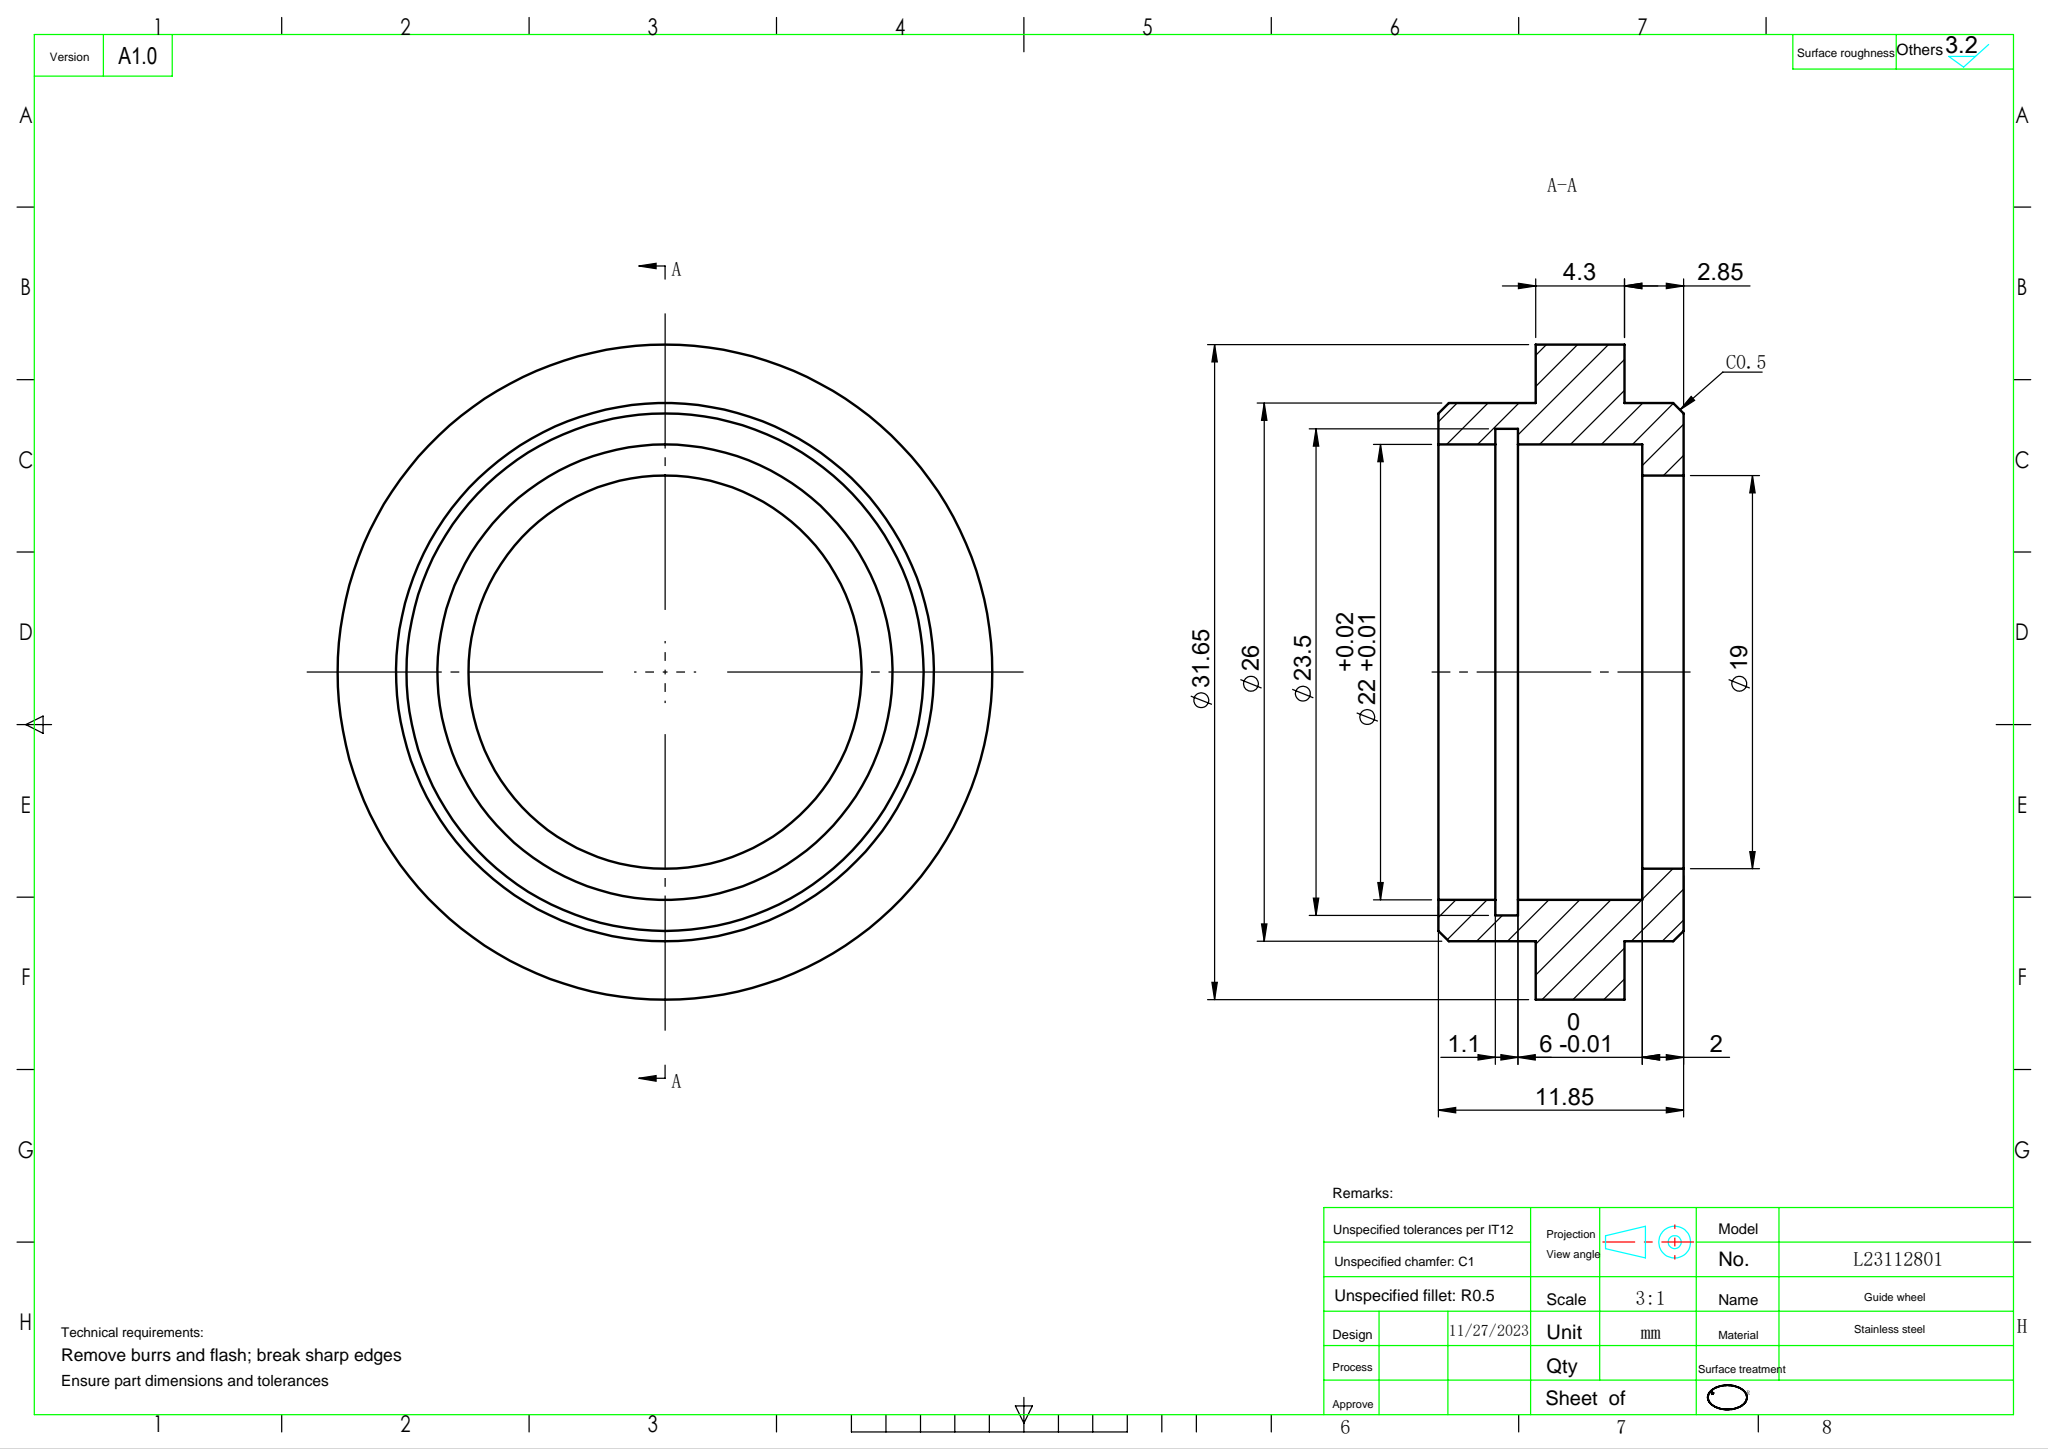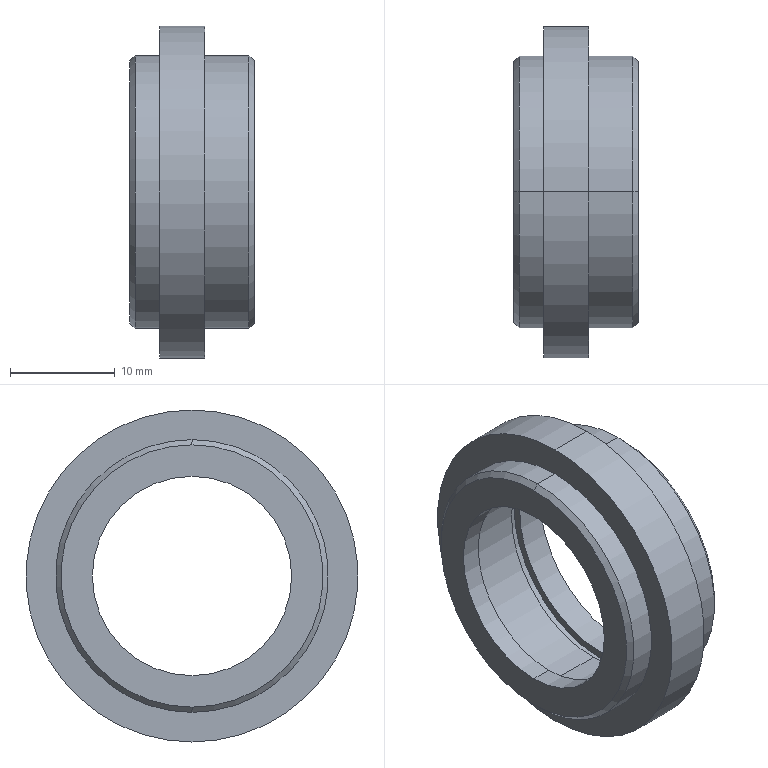Part | SolidWorks | features ICE 2, Chamfer 1, Revolution 1 | 1 solid | 25 faces | box 11.85 x 31.65 x 31.65 mm | volume 3001 mm3 | cylinder 14 | plane 7 | cone 4 | commonest cylinder face diameters 22 x4 26 x4 19 x2 23.5 x2 31.65 x2
STEP:
#1=CARTESIAN_POINT('',(0.,0.,12.5));
#2=VERTEX_POINT('',#1);
#3=CARTESIAN_POINT('',(0.,0.,-12.5));
#4=VERTEX_POINT('',#3);
#5=CARTESIAN_POINT('',(0.,0.,0.));
#6=DIRECTION('',(-1.,0.,0.));
#7=DIRECTION('',(0.,0.,-1.));
#8=AXIS2_PLACEMENT_3D('',#5,#6,#7);
#9=CIRCLE('',#8,12.5);
#10=EDGE_CURVE('',#2,#4,#9,.T.);
#11=ORIENTED_EDGE('',*,*,#10,.F.);
#12=CARTESIAN_POINT('',(0.5,0.,13.));
#13=VERTEX_POINT('',#12);
#14=CARTESIAN_POINT('',(0.,0.,12.5));
#15=DIRECTION('',(0.7071,0.,0.7071));
#16=VECTOR('',#15,1000.);
#17=LINE('',#14,#16);
#18=EDGE_CURVE('',#2,#13,#17,.T.);
#19=ORIENTED_EDGE('',*,*,#18,.T.);
#20=CARTESIAN_POINT('',(0.5,0.,-13.));
#21=VERTEX_POINT('',#20);
#22=CARTESIAN_POINT('',(0.5,0.,0.));
#23=DIRECTION('',(1.,0.,0.));
#24=DIRECTION('',(0.,0.,-1.));
#25=AXIS2_PLACEMENT_3D('',#22,#23,#24);
#26=CIRCLE('',#25,13.);
#27=EDGE_CURVE('',#21,#13,#26,.T.);
#28=ORIENTED_EDGE('',*,*,#27,.F.);
#29=CARTESIAN_POINT('',(0.,0.,-12.5));
#30=DIRECTION('',(0.7071,0.,-0.7071));
#31=VECTOR('',#30,1000.);
#32=LINE('',#29,#31);
#33=EDGE_CURVE('',#4,#21,#32,.T.);
#34=ORIENTED_EDGE('',*,*,#33,.F.);
#35=EDGE_LOOP('',(#11,#19,#28,#34));
#36=FACE_OUTER_BOUND('',#35,.T.);
#37=CARTESIAN_POINT('',(0.,0.,0.));
#38=DIRECTION('',(1.,0.,0.));
#39=DIRECTION('',(0.,0.,-1.));
#40=AXIS2_PLACEMENT_3D('',#37,#38,#39);
#41=CONICAL_SURFACE('',#40,12.5,0.7854);
#42=ADVANCED_FACE('',(#36),#41,.T.);
#43=CARTESIAN_POINT('',(11.85,0.,-12.5));
#44=VERTEX_POINT('',#43);
#45=CARTESIAN_POINT('',(11.85,0.,12.5));
#46=VERTEX_POINT('',#45);
#47=CARTESIAN_POINT('',(11.85,0.,0.));
#48=DIRECTION('',(1.,0.,0.));
#49=DIRECTION('',(0.,0.,1.));
#50=AXIS2_PLACEMENT_3D('',#47,#48,#49);
#51=CIRCLE('',#50,12.5);
#52=EDGE_CURVE('',#44,#46,#51,.T.);
#53=ORIENTED_EDGE('',*,*,#52,.F.);
#54=CARTESIAN_POINT('',(11.35,0.,-13.));
#55=VERTEX_POINT('',#54);
#56=CARTESIAN_POINT('',(11.35,0.,-13.));
#57=DIRECTION('',(-0.7071,0.,-0.7071));
#58=VECTOR('',#57,1000.);
#59=LINE('',#56,#58);
#60=EDGE_CURVE('',#44,#55,#59,.T.);
#61=ORIENTED_EDGE('',*,*,#60,.T.);
#62=CARTESIAN_POINT('',(11.35,0.,13.));
#63=VERTEX_POINT('',#62);
#64=CARTESIAN_POINT('',(11.35,0.,0.));
#65=DIRECTION('',(-1.,0.,0.));
#66=DIRECTION('',(0.,0.,1.));
#67=AXIS2_PLACEMENT_3D('',#64,#65,#66);
#68=CIRCLE('',#67,13.);
#69=EDGE_CURVE('',#63,#55,#68,.T.);
#70=ORIENTED_EDGE('',*,*,#69,.F.);
#71=CARTESIAN_POINT('',(11.35,0.,13.));
#72=DIRECTION('',(-0.7071,0.,0.7071));
#73=VECTOR('',#72,1000.);
#74=LINE('',#71,#73);
#75=EDGE_CURVE('',#46,#63,#74,.T.);
#76=ORIENTED_EDGE('',*,*,#75,.F.);
#77=EDGE_LOOP('',(#53,#61,#70,#76));
#78=FACE_OUTER_BOUND('',#77,.T.);
#79=CARTESIAN_POINT('',(11.35,0.,0.));
#80=DIRECTION('',(-1.,0.,0.));
#81=DIRECTION('',(0.,0.,1.));
#82=AXIS2_PLACEMENT_3D('',#79,#80,#81);
#83=CONICAL_SURFACE('',#82,13.,0.7854);
#84=ADVANCED_FACE('',(#78),#83,.T.);
#85=CARTESIAN_POINT('',(9.1,0.,11.75));
#86=VERTEX_POINT('',#85);
#87=CARTESIAN_POINT('',(9.1,0.,-11.75));
#88=VERTEX_POINT('',#87);
#89=CARTESIAN_POINT('',(9.1,0.,0.));
#90=DIRECTION('',(1.,0.,0.));
#91=DIRECTION('',(0.,0.,-1.));
#92=AXIS2_PLACEMENT_3D('',#89,#90,#91);
#93=CIRCLE('',#92,11.75);
#94=EDGE_CURVE('',#86,#88,#93,.T.);
#95=ORIENTED_EDGE('',*,*,#94,.T.);
#96=CARTESIAN_POINT('',(8.,0.,-11.75));
#97=VERTEX_POINT('',#96);
#98=CARTESIAN_POINT('',(9.1,0.,-11.75));
#99=DIRECTION('',(-1.,0.,0.));
#100=VECTOR('',#99,1000.);
#101=LINE('',#98,#100);
#102=EDGE_CURVE('',#88,#97,#101,.T.);
#103=ORIENTED_EDGE('',*,*,#102,.T.);
#104=CARTESIAN_POINT('',(8.,0.,11.75));
#105=VERTEX_POINT('',#104);
#106=CARTESIAN_POINT('',(8.,0.,0.));
#107=DIRECTION('',(1.,0.,0.));
#108=DIRECTION('',(0.,0.,-1.));
#109=AXIS2_PLACEMENT_3D('',#106,#107,#108);
#110=CIRCLE('',#109,11.75);
#111=EDGE_CURVE('',#105,#97,#110,.T.);
#112=ORIENTED_EDGE('',*,*,#111,.F.);
#113=CARTESIAN_POINT('',(9.1,0.,11.75));
#114=DIRECTION('',(-1.,0.,0.));
#115=VECTOR('',#114,1000.);
#116=LINE('',#113,#115);
#117=EDGE_CURVE('',#86,#105,#116,.T.);
#118=ORIENTED_EDGE('',*,*,#117,.F.);
#119=EDGE_LOOP('',(#95,#103,#112,#118));
#120=FACE_OUTER_BOUND('',#119,.T.);
#121=CARTESIAN_POINT('',(9.1,0.,0.));
#122=DIRECTION('',(-1.,0.,0.));
#123=DIRECTION('',(0.,0.,1.));
#124=AXIS2_PLACEMENT_3D('',#121,#122,#123);
#125=CYLINDRICAL_SURFACE('',#124,11.75);
#126=ADVANCED_FACE('',(#120),#125,.F.);
#127=CARTESIAN_POINT('',(11.85,0.,11.));
#128=VERTEX_POINT('',#127);
#129=CARTESIAN_POINT('',(11.85,0.,-11.));
#130=VERTEX_POINT('',#129);
#131=CARTESIAN_POINT('',(11.85,0.,0.));
#132=DIRECTION('',(1.,0.,0.));
#133=DIRECTION('',(0.,0.,-1.));
#134=AXIS2_PLACEMENT_3D('',#131,#132,#133);
#135=CIRCLE('',#134,11.);
#136=EDGE_CURVE('',#128,#130,#135,.T.);
#137=ORIENTED_EDGE('',*,*,#136,.T.);
#138=CARTESIAN_POINT('',(9.1,0.,-11.));
#139=VERTEX_POINT('',#138);
#140=CARTESIAN_POINT('',(11.85,0.,-11.));
#141=DIRECTION('',(-1.,0.,0.));
#142=VECTOR('',#141,1000.);
#143=LINE('',#140,#142);
#144=EDGE_CURVE('',#130,#139,#143,.T.);
#145=ORIENTED_EDGE('',*,*,#144,.T.);
#146=CARTESIAN_POINT('',(9.1,0.,11.));
#147=VERTEX_POINT('',#146);
#148=CARTESIAN_POINT('',(9.1,0.,0.));
#149=DIRECTION('',(1.,0.,0.));
#150=DIRECTION('',(0.,0.,-1.));
#151=AXIS2_PLACEMENT_3D('',#148,#149,#150);
#152=CIRCLE('',#151,11.);
#153=EDGE_CURVE('',#147,#139,#152,.T.);
#154=ORIENTED_EDGE('',*,*,#153,.F.);
#155=CARTESIAN_POINT('',(11.85,0.,11.));
#156=DIRECTION('',(-1.,0.,0.));
#157=VECTOR('',#156,1000.);
#158=LINE('',#155,#157);
#159=EDGE_CURVE('',#128,#147,#158,.T.);
#160=ORIENTED_EDGE('',*,*,#159,.F.);
#161=EDGE_LOOP('',(#137,#145,#154,#160));
#162=FACE_OUTER_BOUND('',#161,.T.);
#163=CARTESIAN_POINT('',(11.85,0.,0.));
#164=DIRECTION('',(-1.,0.,0.));
#165=DIRECTION('',(0.,0.,1.));
#166=AXIS2_PLACEMENT_3D('',#163,#164,#165);
#167=CYLINDRICAL_SURFACE('',#166,11.);
#168=ADVANCED_FACE('',(#162),#167,.F.);
#169=ORIENTED_EDGE('',*,*,#69,.T.);
#170=CARTESIAN_POINT('',(7.15,0.,-13.));
#171=VERTEX_POINT('',#170);
#172=CARTESIAN_POINT('',(0.,0.,-13.));
#173=DIRECTION('',(-1.,0.,0.));
#174=VECTOR('',#173,1000.);
#175=LINE('',#172,#174);
#176=EDGE_CURVE('',#55,#171,#175,.T.);
#177=ORIENTED_EDGE('',*,*,#176,.T.);
#178=CARTESIAN_POINT('',(7.15,0.,13.));
#179=VERTEX_POINT('',#178);
#180=CARTESIAN_POINT('',(7.15,0.,0.));
#181=DIRECTION('',(-1.,0.,0.));
#182=DIRECTION('',(0.,0.,1.));
#183=AXIS2_PLACEMENT_3D('',#180,#181,#182);
#184=CIRCLE('',#183,13.);
#185=EDGE_CURVE('',#179,#171,#184,.T.);
#186=ORIENTED_EDGE('',*,*,#185,.F.);
#187=CARTESIAN_POINT('',(0.,0.,13.));
#188=DIRECTION('',(-1.,0.,0.));
#189=VECTOR('',#188,1000.);
#190=LINE('',#187,#189);
#191=EDGE_CURVE('',#63,#179,#190,.T.);
#192=ORIENTED_EDGE('',*,*,#191,.F.);
#193=EDGE_LOOP('',(#169,#177,#186,#192));
#194=FACE_OUTER_BOUND('',#193,.T.);
#195=CARTESIAN_POINT('',(0.,0.,0.));
#196=DIRECTION('',(-1.,0.,0.));
#197=DIRECTION('',(0.,0.,1.));
#198=AXIS2_PLACEMENT_3D('',#195,#196,#197);
#199=CYLINDRICAL_SURFACE('',#198,13.);
#200=ADVANCED_FACE('',(#194),#199,.T.);
#201=CARTESIAN_POINT('',(7.15,0.,15.825));
#202=VERTEX_POINT('',#201);
#203=CARTESIAN_POINT('',(7.15,0.,-15.825));
#204=VERTEX_POINT('',#203);
#205=CARTESIAN_POINT('',(7.15,0.,0.));
#206=DIRECTION('',(-1.,0.,0.));
#207=DIRECTION('',(0.,0.,1.));
#208=AXIS2_PLACEMENT_3D('',#205,#206,#207);
#209=CIRCLE('',#208,15.825);
#210=EDGE_CURVE('',#202,#204,#209,.T.);
#211=ORIENTED_EDGE('',*,*,#210,.T.);
#212=CARTESIAN_POINT('',(2.85,0.,-15.825));
#213=VERTEX_POINT('',#212);
#214=CARTESIAN_POINT('',(0.,0.,-15.825));
#215=DIRECTION('',(-1.,0.,0.));
#216=VECTOR('',#215,1000.);
#217=LINE('',#214,#216);
#218=EDGE_CURVE('',#204,#213,#217,.T.);
#219=ORIENTED_EDGE('',*,*,#218,.T.);
#220=CARTESIAN_POINT('',(2.85,0.,15.825));
#221=VERTEX_POINT('',#220);
#222=CARTESIAN_POINT('',(2.85,0.,0.));
#223=DIRECTION('',(-1.,0.,0.));
#224=DIRECTION('',(0.,0.,1.));
#225=AXIS2_PLACEMENT_3D('',#222,#223,#224);
#226=CIRCLE('',#225,15.825);
#227=EDGE_CURVE('',#221,#213,#226,.T.);
#228=ORIENTED_EDGE('',*,*,#227,.F.);
#229=CARTESIAN_POINT('',(0.,0.,15.825));
#230=DIRECTION('',(-1.,0.,0.));
#231=VECTOR('',#230,1000.);
#232=LINE('',#229,#231);
#233=EDGE_CURVE('',#202,#221,#232,.T.);
#234=ORIENTED_EDGE('',*,*,#233,.F.);
#235=EDGE_LOOP('',(#211,#219,#228,#234));
#236=FACE_OUTER_BOUND('',#235,.T.);
#237=CARTESIAN_POINT('',(0.,0.,0.));
#238=DIRECTION('',(-1.,0.,0.));
#239=DIRECTION('',(0.,0.,1.));
#240=AXIS2_PLACEMENT_3D('',#237,#238,#239);
#241=CYLINDRICAL_SURFACE('',#240,15.825);
#242=ADVANCED_FACE('',(#236),#241,.T.);
#243=CARTESIAN_POINT('',(2.85,0.,13.));
#244=VERTEX_POINT('',#243);
#245=CARTESIAN_POINT('',(2.85,0.,-13.));
#246=VERTEX_POINT('',#245);
#247=CARTESIAN_POINT('',(2.85,0.,0.));
#248=DIRECTION('',(-1.,0.,0.));
#249=DIRECTION('',(0.,0.,1.));
#250=AXIS2_PLACEMENT_3D('',#247,#248,#249);
#251=CIRCLE('',#250,13.);
#252=EDGE_CURVE('',#244,#246,#251,.T.);
#253=ORIENTED_EDGE('',*,*,#252,.T.);
#254=CARTESIAN_POINT('',(0.,0.,-13.));
#255=DIRECTION('',(-1.,0.,0.));
#256=VECTOR('',#255,1000.);
#257=LINE('',#254,#256);
#258=EDGE_CURVE('',#246,#21,#257,.T.);
#259=ORIENTED_EDGE('',*,*,#258,.T.);
#260=ORIENTED_EDGE('',*,*,#27,.T.);
#261=CARTESIAN_POINT('',(0.,0.,13.));
#262=DIRECTION('',(-1.,0.,0.));
#263=VECTOR('',#262,1000.);
#264=LINE('',#261,#263);
#265=EDGE_CURVE('',#244,#13,#264,.T.);
#266=ORIENTED_EDGE('',*,*,#265,.F.);
#267=EDGE_LOOP('',(#253,#259,#260,#266));
#268=FACE_OUTER_BOUND('',#267,.T.);
#269=CARTESIAN_POINT('',(0.,0.,0.));
#270=DIRECTION('',(-1.,0.,0.));
#271=DIRECTION('',(0.,0.,1.));
#272=AXIS2_PLACEMENT_3D('',#269,#270,#271);
#273=CYLINDRICAL_SURFACE('',#272,13.);
#274=ADVANCED_FACE('',(#268),#273,.T.);
#275=CARTESIAN_POINT('',(2.,0.,-9.5));
#276=VERTEX_POINT('',#275);
#277=CARTESIAN_POINT('',(2.,0.,9.5));
#278=VERTEX_POINT('',#277);
#279=CARTESIAN_POINT('',(2.,0.,0.));
#280=DIRECTION('',(-1.,0.,0.));
#281=DIRECTION('',(0.,0.,-1.));
#282=AXIS2_PLACEMENT_3D('',#279,#280,#281);
#283=CIRCLE('',#282,9.5);
#284=EDGE_CURVE('',#276,#278,#283,.T.);
#285=ORIENTED_EDGE('',*,*,#284,.F.);
#286=CARTESIAN_POINT('',(0.,0.,-9.5));
#287=VERTEX_POINT('',#286);
#288=CARTESIAN_POINT('',(0.,0.,-9.5));
#289=DIRECTION('',(-1.,0.,0.));
#290=VECTOR('',#289,1000.);
#291=LINE('',#288,#290);
#292=EDGE_CURVE('',#276,#287,#291,.T.);
#293=ORIENTED_EDGE('',*,*,#292,.T.);
#294=CARTESIAN_POINT('',(0.,0.,9.5));
#295=VERTEX_POINT('',#294);
#296=CARTESIAN_POINT('',(0.,0.,0.));
#297=DIRECTION('',(-1.,0.,0.));
#298=DIRECTION('',(0.,0.,1.));
#299=AXIS2_PLACEMENT_3D('',#296,#297,#298);
#300=CIRCLE('',#299,9.5);
#301=EDGE_CURVE('',#287,#295,#300,.T.);
#302=ORIENTED_EDGE('',*,*,#301,.T.);
#303=CARTESIAN_POINT('',(0.,0.,9.5));
#304=DIRECTION('',(-1.,0.,0.));
#305=VECTOR('',#304,1000.);
#306=LINE('',#303,#305);
#307=EDGE_CURVE('',#278,#295,#306,.T.);
#308=ORIENTED_EDGE('',*,*,#307,.F.);
#309=EDGE_LOOP('',(#285,#293,#302,#308));
#310=FACE_OUTER_BOUND('',#309,.T.);
#311=CARTESIAN_POINT('',(0.,0.,0.));
#312=DIRECTION('',(-1.,0.,0.));
#313=DIRECTION('',(0.,0.,1.));
#314=AXIS2_PLACEMENT_3D('',#311,#312,#313);
#315=CYLINDRICAL_SURFACE('',#314,9.5);
#316=ADVANCED_FACE('',(#310),#315,.F.);
#317=CARTESIAN_POINT('',(8.,0.,11.));
#318=VERTEX_POINT('',#317);
#319=CARTESIAN_POINT('',(8.,0.,-11.));
#320=VERTEX_POINT('',#319);
#321=CARTESIAN_POINT('',(8.,0.,0.));
#322=DIRECTION('',(1.,0.,0.));
#323=DIRECTION('',(0.,0.,-1.));
#324=AXIS2_PLACEMENT_3D('',#321,#322,#323);
#325=CIRCLE('',#324,11.);
#326=EDGE_CURVE('',#318,#320,#325,.T.);
#327=ORIENTED_EDGE('',*,*,#326,.T.);
#328=CARTESIAN_POINT('',(2.,0.,-11.));
#329=VERTEX_POINT('',#328);
#330=CARTESIAN_POINT('',(11.85,0.,-11.));
#331=DIRECTION('',(-1.,0.,0.));
#332=VECTOR('',#331,1000.);
#333=LINE('',#330,#332);
#334=EDGE_CURVE('',#320,#329,#333,.T.);
#335=ORIENTED_EDGE('',*,*,#334,.T.);
#336=CARTESIAN_POINT('',(2.,0.,11.));
#337=VERTEX_POINT('',#336);
#338=CARTESIAN_POINT('',(2.,0.,0.));
#339=DIRECTION('',(1.,0.,0.));
#340=DIRECTION('',(0.,0.,-1.));
#341=AXIS2_PLACEMENT_3D('',#338,#339,#340);
#342=CIRCLE('',#341,11.);
#343=EDGE_CURVE('',#337,#329,#342,.T.);
#344=ORIENTED_EDGE('',*,*,#343,.F.);
#345=CARTESIAN_POINT('',(11.85,0.,11.));
#346=DIRECTION('',(-1.,0.,0.));
#347=VECTOR('',#346,1000.);
#348=LINE('',#345,#347);
#349=EDGE_CURVE('',#318,#337,#348,.T.);
#350=ORIENTED_EDGE('',*,*,#349,.F.);
#351=EDGE_LOOP('',(#327,#335,#344,#350));
#352=FACE_OUTER_BOUND('',#351,.T.);
#353=CARTESIAN_POINT('',(11.85,0.,0.));
#354=DIRECTION('',(-1.,0.,0.));
#355=DIRECTION('',(0.,0.,1.));
#356=AXIS2_PLACEMENT_3D('',#353,#354,#355);
#357=CYLINDRICAL_SURFACE('',#356,11.);
#358=ADVANCED_FACE('',(#352),#357,.F.);
#359=ORIENTED_EDGE('',*,*,#334,.F.);
#360=CARTESIAN_POINT('',(8.,0.,0.));
#361=DIRECTION('',(1.,0.,0.));
#362=DIRECTION('',(0.,0.,-1.));
#363=AXIS2_PLACEMENT_3D('',#360,#361,#362);
#364=CIRCLE('',#363,11.);
#365=EDGE_CURVE('',#320,#318,#364,.T.);
#366=ORIENTED_EDGE('',*,*,#365,.T.);
#367=ORIENTED_EDGE('',*,*,#349,.T.);
#368=CARTESIAN_POINT('',(2.,0.,0.));
#369=DIRECTION('',(1.,0.,0.));
#370=DIRECTION('',(0.,0.,-1.));
#371=AXIS2_PLACEMENT_3D('',#368,#369,#370);
#372=CIRCLE('',#371,11.);
#373=EDGE_CURVE('',#329,#337,#372,.T.);
#374=ORIENTED_EDGE('',*,*,#373,.F.);
#375=EDGE_LOOP('',(#359,#366,#367,#374));
#376=FACE_OUTER_BOUND('',#375,.T.);
#377=CARTESIAN_POINT('',(11.85,0.,0.));
#378=DIRECTION('',(-1.,0.,0.));
#379=DIRECTION('',(0.,0.,1.));
#380=AXIS2_PLACEMENT_3D('',#377,#378,#379);
#381=CYLINDRICAL_SURFACE('',#380,11.);
#382=ADVANCED_FACE('',(#376),#381,.F.);
#383=ORIENTED_EDGE('',*,*,#292,.F.);
#384=CARTESIAN_POINT('',(2.,0.,0.));
#385=DIRECTION('',(-1.,0.,0.));
#386=DIRECTION('',(0.,0.,-1.));
#387=AXIS2_PLACEMENT_3D('',#384,#385,#386);
#388=CIRCLE('',#387,9.5);
#389=EDGE_CURVE('',#278,#276,#388,.T.);
#390=ORIENTED_EDGE('',*,*,#389,.F.);
#391=ORIENTED_EDGE('',*,*,#307,.T.);
#392=CARTESIAN_POINT('',(0.,0.,0.));
#393=DIRECTION('',(-1.,0.,0.));
#394=DIRECTION('',(0.,0.,1.));
#395=AXIS2_PLACEMENT_3D('',#392,#393,#394);
#396=CIRCLE('',#395,9.5);
#397=EDGE_CURVE('',#295,#287,#396,.T.);
#398=ORIENTED_EDGE('',*,*,#397,.T.);
#399=EDGE_LOOP('',(#383,#390,#391,#398));
#400=FACE_OUTER_BOUND('',#399,.T.);
#401=CARTESIAN_POINT('',(0.,0.,0.));
#402=DIRECTION('',(-1.,0.,0.));
#403=DIRECTION('',(0.,0.,1.));
#404=AXIS2_PLACEMENT_3D('',#401,#402,#403);
#405=CYLINDRICAL_SURFACE('',#404,9.5);
#406=ADVANCED_FACE('',(#400),#405,.F.);
#407=CARTESIAN_POINT('',(0.,0.,0.));
#408=DIRECTION('',(-1.,0.,0.));
#409=DIRECTION('',(0.,0.,-1.));
#410=AXIS2_PLACEMENT_3D('',#407,#408,#409);
#411=CIRCLE('',#410,12.5);
#412=EDGE_CURVE('',#4,#2,#411,.T.);
#413=ORIENTED_EDGE('',*,*,#412,.T.);
#414=ORIENTED_EDGE('',*,*,#10,.T.);
#415=EDGE_LOOP('',(#413,#414));
#416=FACE_OUTER_BOUND('',#415,.T.);
#417=ORIENTED_EDGE('',*,*,#397,.F.);
#418=ORIENTED_EDGE('',*,*,#301,.F.);
#419=EDGE_LOOP('',(#417,#418));
#420=FACE_BOUND('',#419,.T.);
#421=CARTESIAN_POINT('',(0.,9.5,0.));
#422=DIRECTION('',(1.,0.,0.));
#423=DIRECTION('',(0.,0.,-1.));
#424=AXIS2_PLACEMENT_3D('',#421,#422,#423);
#425=PLANE('',#424);
#426=ADVANCED_FACE('',(#416,#420),#425,.F.);
#427=ORIENTED_EDGE('',*,*,#258,.F.);
#428=CARTESIAN_POINT('',(2.85,0.,0.));
#429=DIRECTION('',(-1.,0.,0.));
#430=DIRECTION('',(0.,0.,1.));
#431=AXIS2_PLACEMENT_3D('',#428,#429,#430);
#432=CIRCLE('',#431,13.);
#433=EDGE_CURVE('',#246,#244,#432,.T.);
#434=ORIENTED_EDGE('',*,*,#433,.T.);
#435=ORIENTED_EDGE('',*,*,#265,.T.);
#436=CARTESIAN_POINT('',(0.5,0.,0.));
#437=DIRECTION('',(1.,0.,0.));
#438=DIRECTION('',(0.,0.,-1.));
#439=AXIS2_PLACEMENT_3D('',#436,#437,#438);
#440=CIRCLE('',#439,13.);
#441=EDGE_CURVE('',#13,#21,#440,.T.);
#442=ORIENTED_EDGE('',*,*,#441,.T.);
#443=EDGE_LOOP('',(#427,#434,#435,#442));
#444=FACE_OUTER_BOUND('',#443,.T.);
#445=CARTESIAN_POINT('',(0.,0.,0.));
#446=DIRECTION('',(-1.,0.,0.));
#447=DIRECTION('',(0.,0.,1.));
#448=AXIS2_PLACEMENT_3D('',#445,#446,#447);
#449=CYLINDRICAL_SURFACE('',#448,13.);
#450=ADVANCED_FACE('',(#444),#449,.T.);
#451=ORIENTED_EDGE('',*,*,#252,.F.);
#452=ORIENTED_EDGE('',*,*,#433,.F.);
#453=EDGE_LOOP('',(#451,#452));
#454=FACE_BOUND('',#453,.T.);
#455=ORIENTED_EDGE('',*,*,#227,.T.);
#456=CARTESIAN_POINT('',(2.85,0.,0.));
#457=DIRECTION('',(-1.,0.,0.));
#458=DIRECTION('',(0.,0.,1.));
#459=AXIS2_PLACEMENT_3D('',#456,#457,#458);
#460=CIRCLE('',#459,15.825);
#461=EDGE_CURVE('',#213,#221,#460,.T.);
#462=ORIENTED_EDGE('',*,*,#461,.T.);
#463=EDGE_LOOP('',(#455,#462));
#464=FACE_OUTER_BOUND('',#463,.T.);
#465=CARTESIAN_POINT('',(2.85,13.,0.));
#466=DIRECTION('',(1.,0.,0.));
#467=DIRECTION('',(0.,0.,-1.));
#468=AXIS2_PLACEMENT_3D('',#465,#466,#467);
#469=PLANE('',#468);
#470=ADVANCED_FACE('',(#454,#464),#469,.F.);
#471=ORIENTED_EDGE('',*,*,#218,.F.);
#472=CARTESIAN_POINT('',(7.15,0.,0.));
#473=DIRECTION('',(-1.,0.,0.));
#474=DIRECTION('',(0.,0.,1.));
#475=AXIS2_PLACEMENT_3D('',#472,#473,#474);
#476=CIRCLE('',#475,15.825);
#477=EDGE_CURVE('',#204,#202,#476,.T.);
#478=ORIENTED_EDGE('',*,*,#477,.T.);
#479=ORIENTED_EDGE('',*,*,#233,.T.);
#480=ORIENTED_EDGE('',*,*,#461,.F.);
#481=EDGE_LOOP('',(#471,#478,#479,#480));
#482=FACE_OUTER_BOUND('',#481,.T.);
#483=CARTESIAN_POINT('',(0.,0.,0.));
#484=DIRECTION('',(-1.,0.,0.));
#485=DIRECTION('',(0.,0.,1.));
#486=AXIS2_PLACEMENT_3D('',#483,#484,#485);
#487=CYLINDRICAL_SURFACE('',#486,15.825);
#488=ADVANCED_FACE('',(#482),#487,.T.);
#489=ORIENTED_EDGE('',*,*,#210,.F.);
#490=ORIENTED_EDGE('',*,*,#477,.F.);
#491=EDGE_LOOP('',(#489,#490));
#492=FACE_OUTER_BOUND('',#491,.T.);
#493=ORIENTED_EDGE('',*,*,#185,.T.);
#494=CARTESIAN_POINT('',(7.15,0.,0.));
#495=DIRECTION('',(-1.,0.,0.));
#496=DIRECTION('',(0.,0.,1.));
#497=AXIS2_PLACEMENT_3D('',#494,#495,#496);
#498=CIRCLE('',#497,13.);
#499=EDGE_CURVE('',#171,#179,#498,.T.);
#500=ORIENTED_EDGE('',*,*,#499,.T.);
#501=EDGE_LOOP('',(#493,#500));
#502=FACE_BOUND('',#501,.T.);
#503=CARTESIAN_POINT('',(7.15,15.825,0.));
#504=DIRECTION('',(-1.,0.,0.));
#505=DIRECTION('',(0.,0.,1.));
#506=AXIS2_PLACEMENT_3D('',#503,#504,#505);
#507=PLANE('',#506);
#508=ADVANCED_FACE('',(#492,#502),#507,.F.);
#509=ORIENTED_EDGE('',*,*,#176,.F.);
#510=CARTESIAN_POINT('',(11.35,0.,0.));
#511=DIRECTION('',(-1.,0.,0.));
#512=DIRECTION('',(0.,0.,1.));
#513=AXIS2_PLACEMENT_3D('',#510,#511,#512);
#514=CIRCLE('',#513,13.);
#515=EDGE_CURVE('',#55,#63,#514,.T.);
#516=ORIENTED_EDGE('',*,*,#515,.T.);
#517=ORIENTED_EDGE('',*,*,#191,.T.);
#518=ORIENTED_EDGE('',*,*,#499,.F.);
#519=EDGE_LOOP('',(#509,#516,#517,#518));
#520=FACE_OUTER_BOUND('',#519,.T.);
#521=CARTESIAN_POINT('',(0.,0.,0.));
#522=DIRECTION('',(-1.,0.,0.));
#523=DIRECTION('',(0.,0.,1.));
#524=AXIS2_PLACEMENT_3D('',#521,#522,#523);
#525=CYLINDRICAL_SURFACE('',#524,13.);
#526=ADVANCED_FACE('',(#520),#525,.T.);
#527=CARTESIAN_POINT('',(11.85,0.,0.));
#528=DIRECTION('',(1.,0.,0.));
#529=DIRECTION('',(0.,0.,1.));
#530=AXIS2_PLACEMENT_3D('',#527,#528,#529);
#531=CIRCLE('',#530,12.5);
#532=EDGE_CURVE('',#46,#44,#531,.T.);
#533=ORIENTED_EDGE('',*,*,#532,.T.);
#534=ORIENTED_EDGE('',*,*,#52,.T.);
#535=EDGE_LOOP('',(#533,#534));
#536=FACE_OUTER_BOUND('',#535,.T.);
#537=ORIENTED_EDGE('',*,*,#136,.F.);
#538=CARTESIAN_POINT('',(11.85,0.,0.));
#539=DIRECTION('',(1.,0.,0.));
#540=DIRECTION('',(0.,0.,-1.));
#541=AXIS2_PLACEMENT_3D('',#538,#539,#540);
#542=CIRCLE('',#541,11.);
#543=EDGE_CURVE('',#130,#128,#542,.T.);
#544=ORIENTED_EDGE('',*,*,#543,.F.);
#545=EDGE_LOOP('',(#537,#544));
#546=FACE_BOUND('',#545,.T.);
#547=CARTESIAN_POINT('',(11.85,13.,0.));
#548=DIRECTION('',(-1.,0.,0.));
#549=DIRECTION('',(0.,0.,1.));
#550=AXIS2_PLACEMENT_3D('',#547,#548,#549);
#551=PLANE('',#550);
#552=ADVANCED_FACE('',(#536,#546),#551,.F.);
#553=ORIENTED_EDGE('',*,*,#343,.T.);
#554=ORIENTED_EDGE('',*,*,#373,.T.);
#555=EDGE_LOOP('',(#553,#554));
#556=FACE_OUTER_BOUND('',#555,.T.);
#557=ORIENTED_EDGE('',*,*,#389,.T.);
#558=ORIENTED_EDGE('',*,*,#284,.T.);
#559=EDGE_LOOP('',(#557,#558));
#560=FACE_BOUND('',#559,.T.);
#561=CARTESIAN_POINT('',(2.,0.,0.));
#562=DIRECTION('',(1.,0.,0.));
#563=DIRECTION('',(0.,0.,-1.));
#564=AXIS2_PLACEMENT_3D('',#561,#562,#563);
#565=PLANE('',#564);
#566=ADVANCED_FACE('',(#556,#560),#565,.T.);
#567=ORIENTED_EDGE('',*,*,#144,.F.);
#568=ORIENTED_EDGE('',*,*,#543,.T.);
#569=ORIENTED_EDGE('',*,*,#159,.T.);
#570=CARTESIAN_POINT('',(9.1,0.,0.));
#571=DIRECTION('',(1.,0.,0.));
#572=DIRECTION('',(0.,0.,-1.));
#573=AXIS2_PLACEMENT_3D('',#570,#571,#572);
#574=CIRCLE('',#573,11.);
#575=EDGE_CURVE('',#139,#147,#574,.T.);
#576=ORIENTED_EDGE('',*,*,#575,.F.);
#577=EDGE_LOOP('',(#567,#568,#569,#576));
#578=FACE_OUTER_BOUND('',#577,.T.);
#579=CARTESIAN_POINT('',(11.85,0.,0.));
#580=DIRECTION('',(-1.,0.,0.));
#581=DIRECTION('',(0.,0.,1.));
#582=AXIS2_PLACEMENT_3D('',#579,#580,#581);
#583=CYLINDRICAL_SURFACE('',#582,11.);
#584=ADVANCED_FACE('',(#578),#583,.F.);
#585=ORIENTED_EDGE('',*,*,#102,.F.);
#586=CARTESIAN_POINT('',(9.1,0.,0.));
#587=DIRECTION('',(1.,0.,0.));
#588=DIRECTION('',(0.,0.,-1.));
#589=AXIS2_PLACEMENT_3D('',#586,#587,#588);
#590=CIRCLE('',#589,11.75);
#591=EDGE_CURVE('',#88,#86,#590,.T.);
#592=ORIENTED_EDGE('',*,*,#591,.T.);
#593=ORIENTED_EDGE('',*,*,#117,.T.);
#594=CARTESIAN_POINT('',(8.,0.,0.));
#595=DIRECTION('',(1.,0.,0.));
#596=DIRECTION('',(0.,0.,-1.));
#597=AXIS2_PLACEMENT_3D('',#594,#595,#596);
#598=CIRCLE('',#597,11.75);
#599=EDGE_CURVE('',#97,#105,#598,.T.);
#600=ORIENTED_EDGE('',*,*,#599,.F.);
#601=EDGE_LOOP('',(#585,#592,#593,#600));
#602=FACE_OUTER_BOUND('',#601,.T.);
#603=CARTESIAN_POINT('',(9.1,0.,0.));
#604=DIRECTION('',(-1.,0.,0.));
#605=DIRECTION('',(0.,0.,1.));
#606=AXIS2_PLACEMENT_3D('',#603,#604,#605);
#607=CYLINDRICAL_SURFACE('',#606,11.75);
#608=ADVANCED_FACE('',(#602),#607,.F.);
#609=ORIENTED_EDGE('',*,*,#153,.T.);
#610=ORIENTED_EDGE('',*,*,#575,.T.);
#611=EDGE_LOOP('',(#609,#610));
#612=FACE_BOUND('',#611,.T.);
#613=ORIENTED_EDGE('',*,*,#94,.F.);
#614=ORIENTED_EDGE('',*,*,#591,.F.);
#615=EDGE_LOOP('',(#613,#614));
#616=FACE_OUTER_BOUND('',#615,.T.);
#617=CARTESIAN_POINT('',(9.1,0.,0.));
#618=DIRECTION('',(1.,0.,0.));
#619=DIRECTION('',(0.,0.,-1.));
#620=AXIS2_PLACEMENT_3D('',#617,#618,#619);
#621=PLANE('',#620);
#622=ADVANCED_FACE('',(#612,#616),#621,.F.);
#623=ORIENTED_EDGE('',*,*,#326,.F.);
#624=ORIENTED_EDGE('',*,*,#365,.F.);
#625=EDGE_LOOP('',(#623,#624));
#626=FACE_BOUND('',#625,.T.);
#627=ORIENTED_EDGE('',*,*,#111,.T.);
#628=ORIENTED_EDGE('',*,*,#599,.T.);
#629=EDGE_LOOP('',(#627,#628));
#630=FACE_OUTER_BOUND('',#629,.T.);
#631=CARTESIAN_POINT('',(8.,0.,0.));
#632=DIRECTION('',(1.,0.,0.));
#633=DIRECTION('',(0.,0.,-1.));
#634=AXIS2_PLACEMENT_3D('',#631,#632,#633);
#635=PLANE('',#634);
#636=ADVANCED_FACE('',(#626,#630),#635,.T.);
#637=ORIENTED_EDGE('',*,*,#60,.F.);
#638=ORIENTED_EDGE('',*,*,#532,.F.);
#639=ORIENTED_EDGE('',*,*,#75,.T.);
#640=ORIENTED_EDGE('',*,*,#515,.F.);
#641=EDGE_LOOP('',(#637,#638,#639,#640));
#642=FACE_OUTER_BOUND('',#641,.T.);
#643=CARTESIAN_POINT('',(11.35,0.,0.));
#644=DIRECTION('',(-1.,0.,0.));
#645=DIRECTION('',(0.,0.,1.));
#646=AXIS2_PLACEMENT_3D('',#643,#644,#645);
#647=CONICAL_SURFACE('',#646,13.,0.7854);
#648=ADVANCED_FACE('',(#642),#647,.T.);
#649=ORIENTED_EDGE('',*,*,#18,.F.);
#650=ORIENTED_EDGE('',*,*,#412,.F.);
#651=ORIENTED_EDGE('',*,*,#33,.T.);
#652=ORIENTED_EDGE('',*,*,#441,.F.);
#653=EDGE_LOOP('',(#649,#650,#651,#652));
#654=FACE_OUTER_BOUND('',#653,.T.);
#655=CARTESIAN_POINT('',(0.,0.,0.));
#656=DIRECTION('',(1.,0.,0.));
#657=DIRECTION('',(0.,0.,-1.));
#658=AXIS2_PLACEMENT_3D('',#655,#656,#657);
#659=CONICAL_SURFACE('',#658,12.5,0.7854);
#660=ADVANCED_FACE('',(#654),#659,.T.);
#661=CLOSED_SHELL('',(#42,#84,#126,#168,#200,#242,#274,#316,#358,#382,#406,#426,#450,#470,#488,#508,#526,#552,#566,#584,#608,#622,#636,#648,#660));
#662=MANIFOLD_SOLID_BREP('',#661);
#663=CARTESIAN_POINT('',(0.,0.,0.));
#664=DIRECTION('',(0.,0.,1.));
#665=DIRECTION('',(1.,0.,0.));
#666=AXIS2_PLACEMENT_3D('',#663,#664,#665);
#667=(LENGTH_UNIT()NAMED_UNIT(*)SI_UNIT(.MILLI.,.METRE.));
#668=UNCERTAINTY_MEASURE_WITH_UNIT(LENGTH_MEASURE(0.00001),#667,'','');
#669=(NAMED_UNIT(*)PLANE_ANGLE_UNIT()SI_UNIT($,.RADIAN.));
#670=(NAMED_UNIT(*)SI_UNIT($,.STERADIAN.)SOLID_ANGLE_UNIT());
#671=(GEOMETRIC_REPRESENTATION_CONTEXT(3)GLOBAL_UNCERTAINTY_ASSIGNED_CONTEXT((#668))GLOBAL_UNIT_ASSIGNED_CONTEXT((#667,#669,#670))REPRESENTATION_CONTEXT('',''));
#672=ADVANCED_BREP_SHAPE_REPRESENTATION('',(#662,#666),#671);